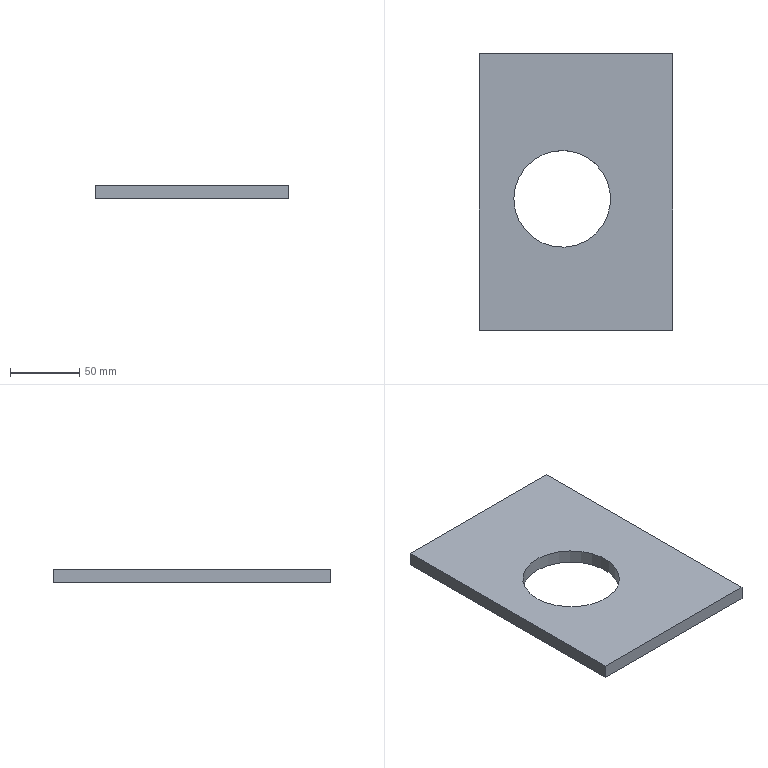Part | NX | features solid 2 | 1 solid | 7 faces | box 140 x 200 x 10 mm | volume 241515 mm3 | plane 6 | cylinder 1 | commonest cylinder face diameters 70 x1
STEP:
#1=CARTESIAN_POINT('',(-1220.,-195.,-460.));
#2=VERTEX_POINT('',#1);
#3=CARTESIAN_POINT('',(-1360.,-195.,-460.));
#4=VERTEX_POINT('',#3);
#5=CARTESIAN_POINT('',(-1120.,-195.,-460.));
#6=DIRECTION('',(-1.,0.,0.));
#7=VECTOR('',#6,1000.);
#8=LINE('',#5,#7);
#9=EDGE_CURVE('',#2,#4,#8,.T.);
#10=ORIENTED_EDGE('',*,*,#9,.T.);
#11=CARTESIAN_POINT('',(-1360.,-195.,-450.));
#12=VERTEX_POINT('',#11);
#13=CARTESIAN_POINT('',(-1360.,-195.,-450.));
#14=DIRECTION('',(0.,0.,-1.));
#15=VECTOR('',#14,1000.);
#16=LINE('',#13,#15);
#17=EDGE_CURVE('',#12,#4,#16,.T.);
#18=ORIENTED_EDGE('',*,*,#17,.F.);
#19=CARTESIAN_POINT('',(-1220.,-195.,-450.));
#20=VERTEX_POINT('',#19);
#21=CARTESIAN_POINT('',(-1120.,-195.,-450.));
#22=DIRECTION('',(-1.,0.,0.));
#23=VECTOR('',#22,1000.);
#24=LINE('',#21,#23);
#25=EDGE_CURVE('',#20,#12,#24,.T.);
#26=ORIENTED_EDGE('',*,*,#25,.F.);
#27=CARTESIAN_POINT('',(-1220.,-195.,-450.));
#28=DIRECTION('',(0.,0.,-1.));
#29=VECTOR('',#28,1000.);
#30=LINE('',#27,#29);
#31=EDGE_CURVE('',#20,#2,#30,.T.);
#32=ORIENTED_EDGE('',*,*,#31,.T.);
#33=EDGE_LOOP('',(#10,#18,#26,#32));
#34=FACE_BOUND('',#33,.T.);
#35=CARTESIAN_POINT('',(-1120.,-195.,-450.));
#36=DIRECTION('',(0.,-1.,0.));
#37=DIRECTION('',(1.,0.,0.));
#38=AXIS2_PLACEMENT_3D('',#35,#36,#37);
#39=PLANE('',#38);
#40=ADVANCED_FACE('',(#34),#39,.F.);
#41=CARTESIAN_POINT('',(-1220.,-395.,-460.));
#42=VERTEX_POINT('',#41);
#43=CARTESIAN_POINT('',(-1220.,-220.,-460.));
#44=DIRECTION('',(0.,-1.,0.));
#45=VECTOR('',#44,1000.);
#46=LINE('',#43,#45);
#47=EDGE_CURVE('',#2,#42,#46,.T.);
#48=ORIENTED_EDGE('',*,*,#47,.F.);
#49=ORIENTED_EDGE('',*,*,#31,.F.);
#50=CARTESIAN_POINT('',(-1220.,-395.,-450.));
#51=VERTEX_POINT('',#50);
#52=CARTESIAN_POINT('',(-1220.,-220.,-450.));
#53=DIRECTION('',(0.,-1.,0.));
#54=VECTOR('',#53,1000.);
#55=LINE('',#52,#54);
#56=EDGE_CURVE('',#20,#51,#55,.T.);
#57=ORIENTED_EDGE('',*,*,#56,.T.);
#58=CARTESIAN_POINT('',(-1220.,-395.,-450.));
#59=DIRECTION('',(0.,0.,-1.));
#60=VECTOR('',#59,1000.);
#61=LINE('',#58,#60);
#62=EDGE_CURVE('',#51,#42,#61,.T.);
#63=ORIENTED_EDGE('',*,*,#62,.T.);
#64=EDGE_LOOP('',(#48,#49,#57,#63));
#65=FACE_BOUND('',#64,.T.);
#66=CARTESIAN_POINT('',(-1220.,-220.,-450.));
#67=DIRECTION('',(1.,0.,0.));
#68=DIRECTION('',(0.,1.,0.));
#69=AXIS2_PLACEMENT_3D('',#66,#67,#68);
#70=PLANE('',#69);
#71=ADVANCED_FACE('',(#65),#70,.T.);
#72=CARTESIAN_POINT('',(-1360.,-395.,-460.));
#73=VERTEX_POINT('',#72);
#74=CARTESIAN_POINT('',(-1400.,-395.,-460.));
#75=DIRECTION('',(-1.,0.,0.));
#76=VECTOR('',#75,1000.);
#77=LINE('',#74,#76);
#78=EDGE_CURVE('',#42,#73,#77,.T.);
#79=ORIENTED_EDGE('',*,*,#78,.F.);
#80=ORIENTED_EDGE('',*,*,#62,.F.);
#81=CARTESIAN_POINT('',(-1360.,-395.,-450.));
#82=VERTEX_POINT('',#81);
#83=CARTESIAN_POINT('',(-1400.,-395.,-450.));
#84=DIRECTION('',(-1.,0.,0.));
#85=VECTOR('',#84,1000.);
#86=LINE('',#83,#85);
#87=EDGE_CURVE('',#51,#82,#86,.T.);
#88=ORIENTED_EDGE('',*,*,#87,.T.);
#89=CARTESIAN_POINT('',(-1360.,-395.,-450.));
#90=DIRECTION('',(0.,0.,-1.));
#91=VECTOR('',#90,1000.);
#92=LINE('',#89,#91);
#93=EDGE_CURVE('',#82,#73,#92,.T.);
#94=ORIENTED_EDGE('',*,*,#93,.T.);
#95=EDGE_LOOP('',(#79,#80,#88,#94));
#96=FACE_BOUND('',#95,.T.);
#97=CARTESIAN_POINT('',(-1400.,-395.,-450.));
#98=DIRECTION('',(0.,-1.,0.));
#99=DIRECTION('',(1.,0.,0.));
#100=AXIS2_PLACEMENT_3D('',#97,#98,#99);
#101=PLANE('',#100);
#102=ADVANCED_FACE('',(#96),#101,.T.);
#103=CARTESIAN_POINT('',(-1360.,779.99,-460.));
#104=DIRECTION('',(0.,-1.,0.));
#105=VECTOR('',#104,1000.);
#106=LINE('',#103,#105);
#107=EDGE_CURVE('',#4,#73,#106,.T.);
#108=ORIENTED_EDGE('',*,*,#107,.T.);
#109=ORIENTED_EDGE('',*,*,#93,.F.);
#110=CARTESIAN_POINT('',(-1360.,779.99,-450.));
#111=DIRECTION('',(0.,-1.,0.));
#112=VECTOR('',#111,1000.);
#113=LINE('',#110,#112);
#114=EDGE_CURVE('',#12,#82,#113,.T.);
#115=ORIENTED_EDGE('',*,*,#114,.F.);
#116=ORIENTED_EDGE('',*,*,#17,.T.);
#117=EDGE_LOOP('',(#108,#109,#115,#116));
#118=FACE_BOUND('',#117,.T.);
#119=CARTESIAN_POINT('',(-1360.,779.99,-450.));
#120=DIRECTION('',(1.,0.,0.));
#121=DIRECTION('',(0.,0.,-1.));
#122=AXIS2_PLACEMENT_3D('',#119,#120,#121);
#123=PLANE('',#122);
#124=ADVANCED_FACE('',(#118),#123,.F.);
#125=CARTESIAN_POINT('',(-1335.,-300.,-450.));
#126=VERTEX_POINT('',#125);
#127=CARTESIAN_POINT('',(-1300.,-300.,-450.));
#128=DIRECTION('',(0.,0.,-1.));
#129=DIRECTION('',(-1.,0.,0.));
#130=AXIS2_PLACEMENT_3D('',#127,#128,#129);
#131=CIRCLE('',#130,35.);
#132=EDGE_CURVE('',#126,#126,#131,.T.);
#133=ORIENTED_EDGE('',*,*,#132,.F.);
#134=EDGE_LOOP('',(#133));
#135=FACE_BOUND('',#134,.T.);
#136=CARTESIAN_POINT('',(-1335.,-300.,-460.));
#137=VERTEX_POINT('',#136);
#138=CARTESIAN_POINT('',(-1300.,-300.,-460.));
#139=DIRECTION('',(0.,0.,-1.));
#140=DIRECTION('',(-1.,0.,0.));
#141=AXIS2_PLACEMENT_3D('',#138,#139,#140);
#142=CIRCLE('',#141,35.);
#143=EDGE_CURVE('',#137,#137,#142,.T.);
#144=ORIENTED_EDGE('',*,*,#143,.T.);
#145=EDGE_LOOP('',(#144));
#146=FACE_BOUND('',#145,.T.);
#147=CARTESIAN_POINT('',(-1300.,-300.,-450.));
#148=DIRECTION('',(0.,0.,-1.));
#149=DIRECTION('',(-1.,0.,0.));
#150=AXIS2_PLACEMENT_3D('',#147,#148,#149);
#151=CYLINDRICAL_SURFACE('',#150,35.);
#152=ADVANCED_FACE('',(#135,#146),#151,.F.);
#153=ORIENTED_EDGE('',*,*,#25,.T.);
#154=ORIENTED_EDGE('',*,*,#114,.T.);
#155=ORIENTED_EDGE('',*,*,#87,.F.);
#156=ORIENTED_EDGE('',*,*,#56,.F.);
#157=EDGE_LOOP('',(#153,#154,#155,#156));
#158=FACE_BOUND('',#157,.T.);
#159=ORIENTED_EDGE('',*,*,#132,.T.);
#160=EDGE_LOOP('',(#159));
#161=FACE_BOUND('',#160,.T.);
#162=CARTESIAN_POINT('',(-1400.,-220.,-450.));
#163=DIRECTION('',(0.,0.,-1.));
#164=DIRECTION('',(-1.,0.,0.));
#165=AXIS2_PLACEMENT_3D('',#162,#163,#164);
#166=PLANE('',#165);
#167=ADVANCED_FACE('',(#158,#161),#166,.F.);
#168=ORIENTED_EDGE('',*,*,#9,.F.);
#169=ORIENTED_EDGE('',*,*,#47,.T.);
#170=ORIENTED_EDGE('',*,*,#78,.T.);
#171=ORIENTED_EDGE('',*,*,#107,.F.);
#172=EDGE_LOOP('',(#168,#169,#170,#171));
#173=FACE_BOUND('',#172,.T.);
#174=ORIENTED_EDGE('',*,*,#143,.F.);
#175=EDGE_LOOP('',(#174));
#176=FACE_BOUND('',#175,.T.);
#177=CARTESIAN_POINT('',(-1400.,-220.,-460.));
#178=DIRECTION('',(0.,0.,-1.));
#179=DIRECTION('',(-1.,0.,0.));
#180=AXIS2_PLACEMENT_3D('',#177,#178,#179);
#181=PLANE('',#180);
#182=ADVANCED_FACE('',(#173,#176),#181,.T.);
#183=CLOSED_SHELL('',(#40,#71,#102,#124,#152,#167,#182));
#184=MANIFOLD_SOLID_BREP('',#183);
#185=(LENGTH_UNIT()NAMED_UNIT(*)SI_UNIT(.MILLI.,.METRE.));
#186=UNCERTAINTY_MEASURE_WITH_UNIT(LENGTH_MEASURE(0.00001),#185,'','');
#187=(NAMED_UNIT(*)PLANE_ANGLE_UNIT()SI_UNIT($,.RADIAN.));
#188=(NAMED_UNIT(*)SI_UNIT($,.STERADIAN.)SOLID_ANGLE_UNIT());
#189=(GEOMETRIC_REPRESENTATION_CONTEXT(3)GLOBAL_UNCERTAINTY_ASSIGNED_CONTEXT((#186))GLOBAL_UNIT_ASSIGNED_CONTEXT((#185,#187,#188))REPRESENTATION_CONTEXT('',''));
#190=ADVANCED_BREP_SHAPE_REPRESENTATION('',(#184),#189);